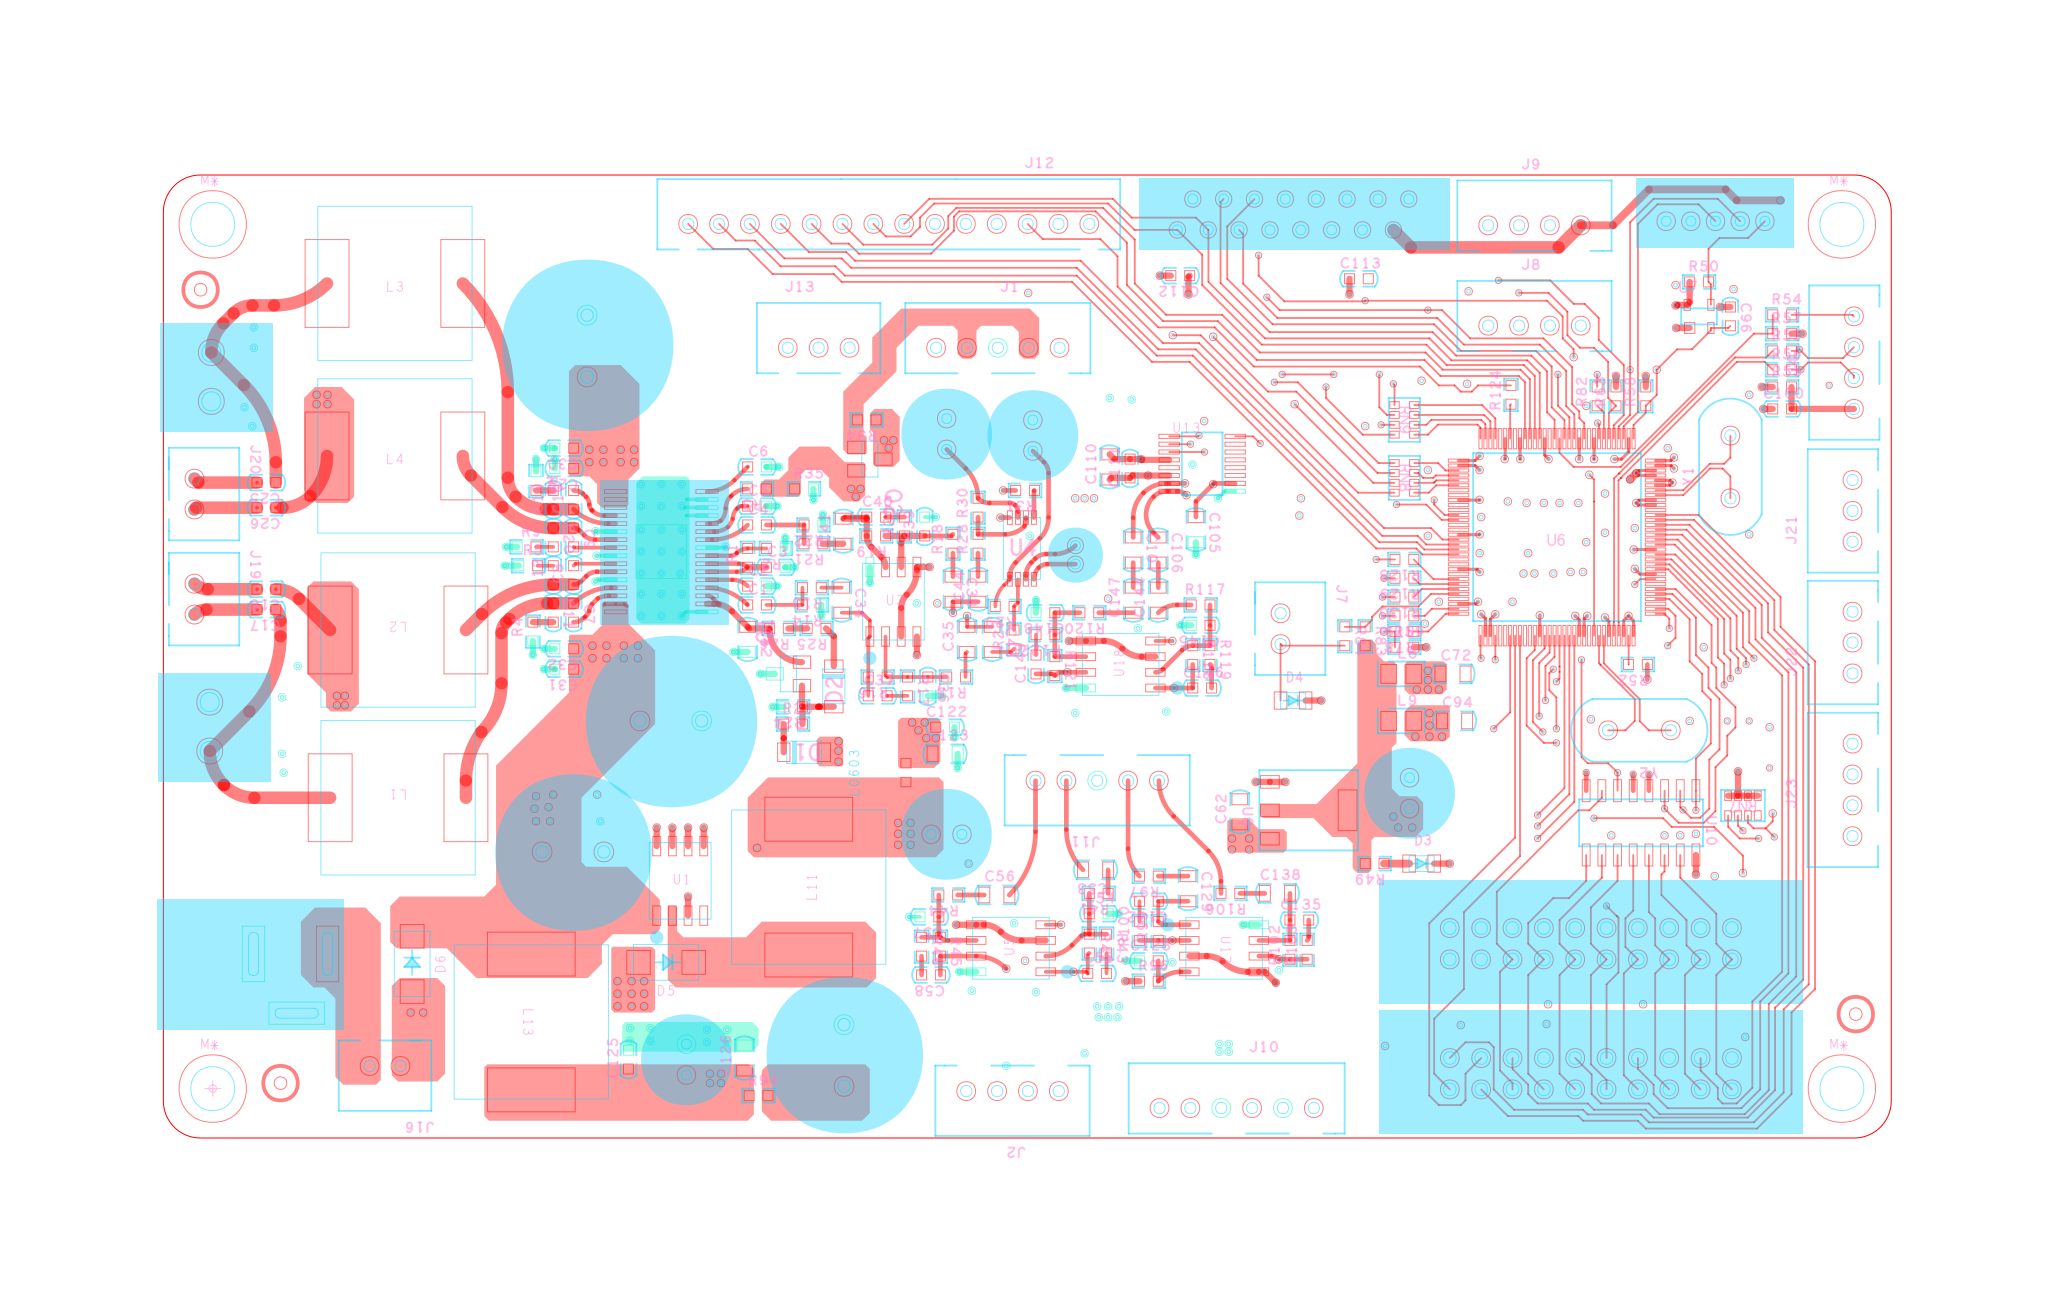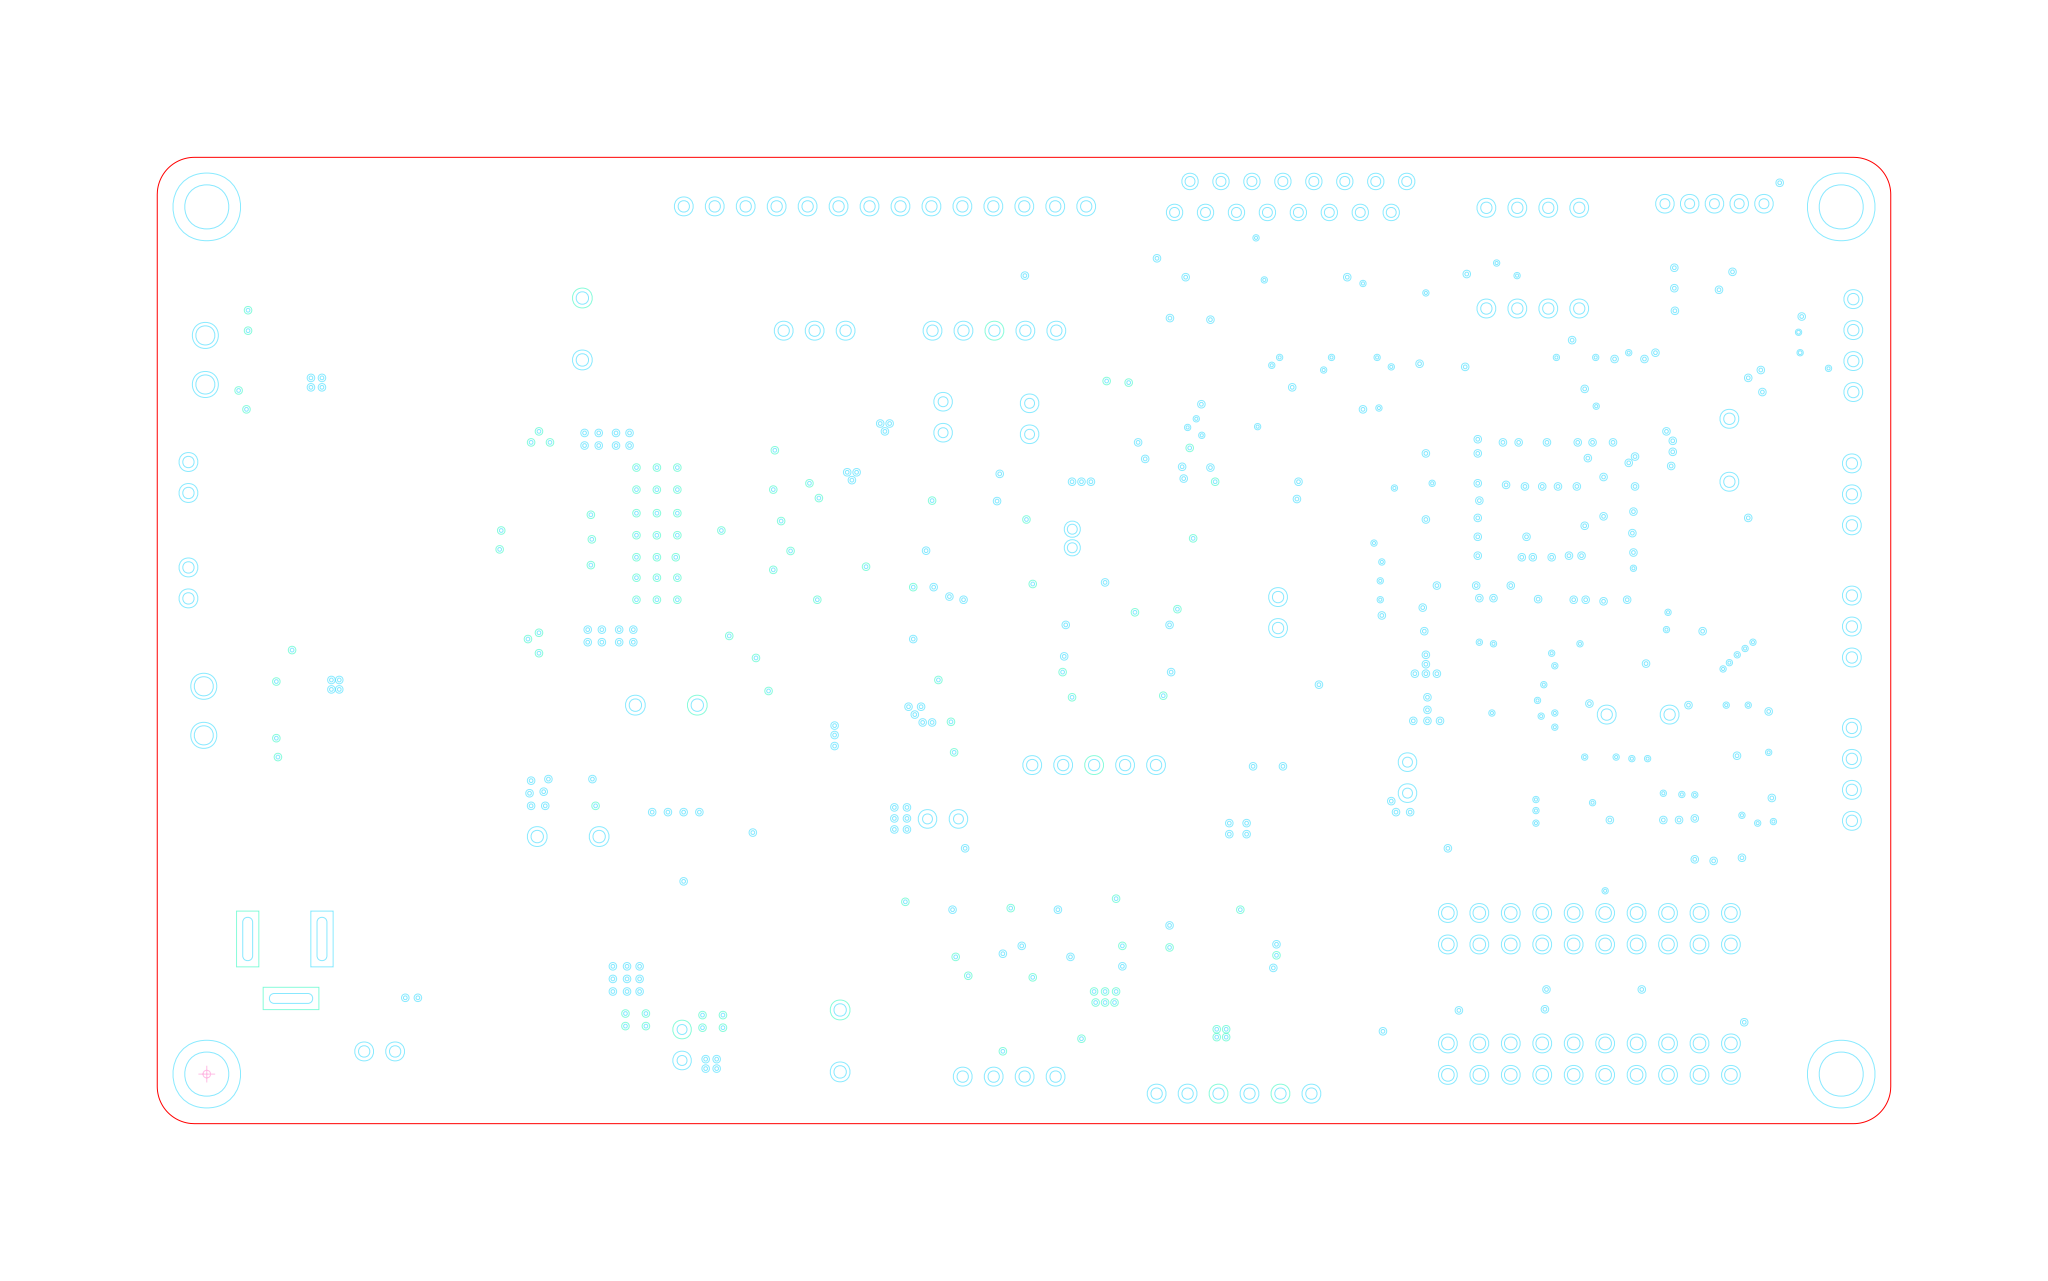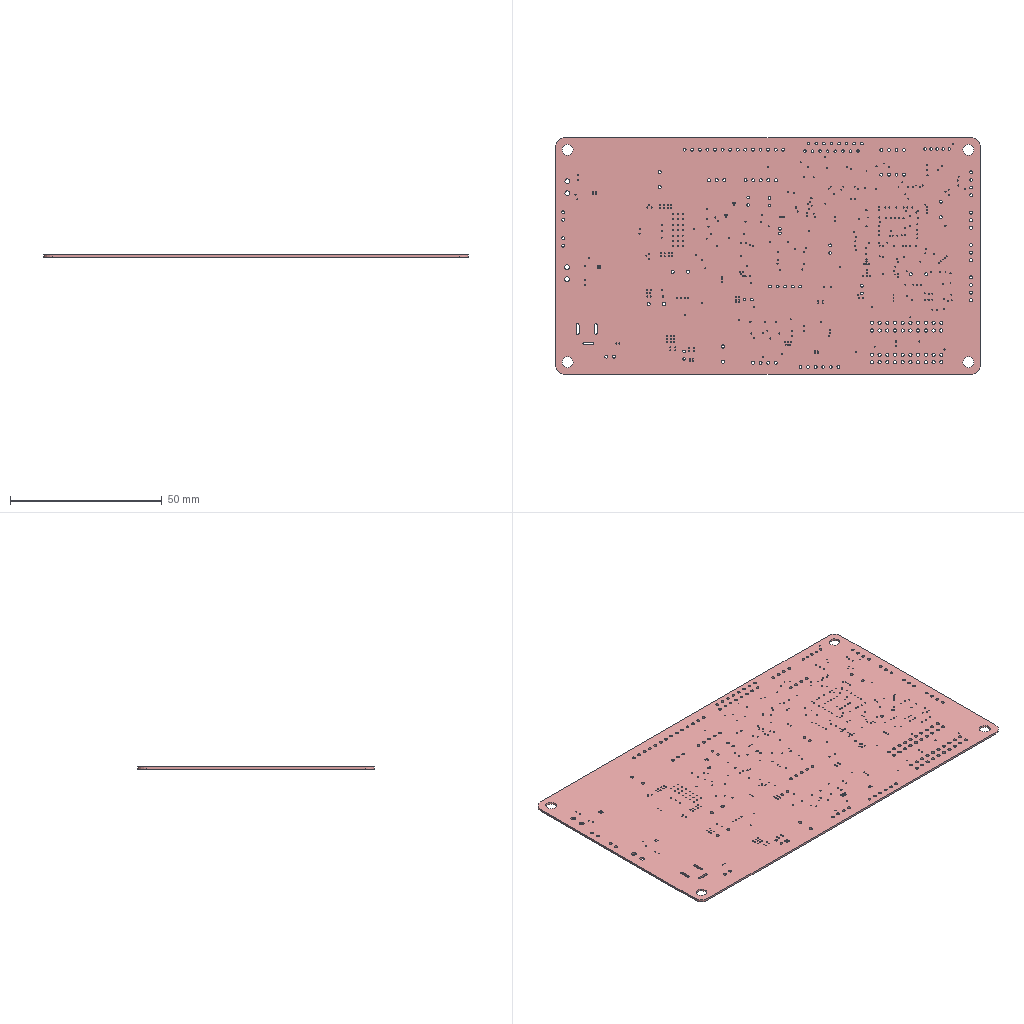Circuit board layout | Cadence Allegro | box 140 x 78 x 0.7 mm
Layer stack:
# Cadence Allegro layer stack of  (unit mm; from the constraint file cross-section; dielectric type: 0 not recorded (Allegro does not mark core vs prepreg), 3 surface material)
index,name,kind,layer,copper_thickness_mm,dielectric_type,dielectric_thickness_mm,dielectric_material,dielectric_constant
0,Top Surface,other,,,,,,
1,TOP,copper,TOP,0.0305,,,,
2,Dielectric1,dielectric,,,0,0.2032,FR-4,4.5
3,L2GND,copper,L2GND,0.0305,,,,
4,Dielectric2,dielectric,,,0,0.2032,FR-4,4.5
5,L3VCC,copper,L3VCC,0.0305,,,,
6,Dielectric3,dielectric,,,0,0.2032,FR-4,4.5
7,BOTTOM,copper,BOTTOM,0.0305,,,,
8,Bottom Surface,other,,,,,,
# drill layer pairs: low layer,high layer
drill_pair,TOP,BOTTOM
Part placement:
REFDES,COMP_VALUE,SYM_NAME,SYM_X,SYM_Y,SYM_ROTATE,SYM_MIRROR
C1,1nF,C0603,1736.220,1542.520,0.000,NO
C2,1nF,C0603,1736.220,1602.520,0.000,NO
C3,1nF,C0603,1796.220,1662.520,0.000,NO
C4,1nF,C0603,1736.220,1797.520,0.000,NO
C5,1nF,C0603,1736.220,1857.520,0.000,NO
C6,1nF,C0603,1736.220,1982.520,0.000,NO
C7,220nF/50V,C0603,1151.220,1517.520,270.000,NO
C8,220nF/50V,C0603,1151.220,1637.520,90.000,NO
C9,220nF/50V,C0603,1151.220,1757.520,270.000,NO
C10,220nF/50V,C0603,1151.220,1877.520,90.000,NO
C11,33pF/50V,C0603,1086.220,1517.520,270.000,NO
C12,33pF/50V,C0603,1086.220,1637.520,90.000,NO
C13,680nF,C0603,256.220,1097.520,90.000,YES
C14,680nF,C0603,256.220,1217.520,90.000,YES
C15,10nF/50V,C0603,301.220,1007.520,0.000,YES
C16,10nF/50V,C0603,301.220,1307.520,0.000,YES
C17,DNP-3.3uF/50V,C0603,171.220,1527.520,180.000,NO
C18,DNP-3.3uF/50V,C0603,171.220,1592.520,180.000,NO
C19,33pF/50V,C0603,1086.220,1877.520,90.000,NO
C20,33pF/50V,C0603,1086.220,1757.520,270.000,NO
C21,680nF,C0603,166.220,2332.520,270.000,YES
C22,680nF,C0603,166.220,2202.520,270.000,YES
C23,10nF/50V,C0603,196.220,2427.520,0.000,YES
C24,10nF/50V,C0603,196.220,2112.520,0.000,YES
C25,DNP-3.3uF/50V,C0603,171.220,1932.520,180.000,NO
C26,DNP-3.3uF/50V,C0603,171.220,1852.520,180.000,NO
C27,1000uF/35V,CAP_13X20MM,1194.251,2367.914,90.000,NO
C28,1000uF/35V,CAP_13X20MM,1461.220,1172.520,0.000,NO
C29,0.1uF,C0603,1121.220,1977.520,180.000,NO
C30,0.1uF,C0603,1121.220,2042.520,180.000,NO
C31,1nF,C0603,1121.220,1337.520,180.000,NO
C32,1nF,C0603,1121.220,1402.520,180.000,NO
C33,0.1uF,C0603,2246.220,1472.520,90.000,YES
C34,10uF,C0805,2006.220,1557.520,270.000,NO
C35,10uF,C0805,2406.220,1432.520,90.000,NO
C36,1nF,C0603,2281.220,1282.520,270.000,NO
C37,100pF,C0603,2121.220,1252.520,0.000,NO
C38,10uF,C0805,2361.220,1592.520,270.000,NO
C39,1nF,C0603,2271.220,1792.520,90.000,NO
C40,100pF,C0603,2116.220,1822.520,0.000,NO
C41,10uF,C0805,2011.220,1777.520,90.000,NO
C42,10uF,C0805,1706.220,1432.520,270.000,NO
C43,10uF,C0805,2486.220,1432.520,270.000,NO
C44,10uF,C0805,2441.220,1592.520,90.000,NO
C45,100uF/10V,CAP_6P3X11MM,2616.220,2082.520,90.000,NO
C46,100uF/10V,CAP_6P3X11MM,2341.220,2087.520,90.000,NO
C47,1uF,C0603,2576.220,1822.520,180.000,YES
C48,4.7uF/35V,CAP_4X7MM,2752.007,1702.126,270.000,NO
C49,0.1uF,C0603,2141.220,1977.520,90.000,YES
C50,10uF,C0805,2531.220,292.520,270.000,YES
C51,0.1uF,C0603,2626.220,527.520,180.000,YES
C52,10uF,C0805,2746.220,287.520,270.000,YES
C53,10uF,C0805,2816.220,697.520,180.000,NO
C54,1nF,C0603,2826.220,557.520,0.000,NO
C55,100pF,C0603,2821.220,367.520,0.000,NO
C56,10uF,C0805,2501.220,617.520,0.000,NO
C57,1nF,C0603,2286.220,547.520,180.000,NO
C58,100pF,C0603,2291.220,362.520,180.000,NO
C59,DNP,C0603,2716.220,112.520,180.000,YES
C60,DNP,C0603,2501.220,112.520,180.000,YES
C61,0.1uF,C0603,3276.220,877.520,270.000,YES
C62,10uF,C0805,3276.220,882.520,90.000,NO
C63,0.1uF,C0603,3921.220,937.520,270.000,YES
C64,100uF,CAP_6P3X11MM,3817.795,942.126,90.000,NO
C65,0.1uF,C0603,4131.220,1937.520,90.000,YES
C66,10nF,C0603,4356.220,1937.520,90.000,YES
C67,10uF,C0805,3981.220,1597.520,0.000,YES
C68,0.1uF,C0603,4296.220,1937.522,90.000,YES
C69,10nF,C0603,4081.220,1992.520,270.000,YES
C70,0.1uF,C0603,3956.220,1322.520,180.000,YES
C71,10nF,C0603,4081.220,1852.520,90.000,YES
C72,10uF,C0805,3956.220,1322.520,0.000,NO
C73,0.1uF,C0603,4001.220,1737.520,90.000,YES
C74,10uF,C0805,4651.220,1747.520,270.000,YES
C75,0.1uF,C0603,4246.220,1937.520,90.000,YES
C76,10nF,C0603,4591.220,1997.520,180.000,YES
C77,0.1uF,C0603,4191.220,1937.520,90.000,YES
C78,10nF,C0603,4116.220,1587.520,180.000,YES
C79,0.1uF,C0603,4471.220,1742.520,0.000,YES
C80,0.1uF,C0603,4276.220,1577.520,270.000,YES
C81,10nF,C0603,4331.220,1577.520,270.000,YES
C82,10uF,C0805,4121.220,1707.520,180.000,YES
C83,0.1uF,C0603,4116.220,1642.520,180.000,YES
C84,10nF,C0603,4591.220,1917.520,180.000,YES
C85,10uF,C0805,4581.220,1747.520,270.000,YES
C86,10uF,C0805,4451.220,1672.520,0.000,YES
C87,0.1uF,C0603,4386.220,1577.520,270.000,YES
C88,0.1uF,C0603,4451.220,2052.520,180.000,YES
C89,10nF,C0603,4471.220,1867.520,0.000,YES
C90,0.1uF,C0603,4471.220,1807.520,0.000,YES
C91,0.1uF,C0603,4216.220,1577.520,270.000,YES
C92,0.1uF,C0603,4696.220,1997.520,270.000,YES
C93,0.1uF,C0603,4441.220,1577.520,270.000,YES
C94,10uF,C0805,3961.220,1172.520,0.000,NO
C95,0.1uF,C0603,4066.220,1472.520,180.000,YES
C96,0.1uF,C0603,4841.220,2462.520,270.000,NO
C97,0.1uF,C0603,4701.220,2462.520,90.000,YES
C98,0.1uF,C0603,4781.220,2612.520,270.000,YES
C99,10uF,C0805,4711.220,2602.520,90.000,YES
C100,0.1uF,C0603,5006.220,2167.520,0.000,NO
C101,0.1uF,C0603,4761.220,642.520,0.000,YES
C102,0.1uF,C0603,4966.220,1087.520,90.000,YES
C103,10uF,C0805,2861.220,2127.520,270.000,YES
C104,0.1uF,C0603,2931.220,2127.520,270.000,YES
C105,10uF,C0805,3136.220,1782.520,270.000,NO
C106,10uF,C0805,3016.220,1717.520,270.000,NO
C107,10uF,C0805,2936.220,1717.520,270.000,NO
C108,10uF,C0805,2862.535,1982.520,270.000,YES
C109,0.1uF,C0603,2927.535,1977.520,270.000,YES
C110,10uF,C0805,2861.220,1982.520,90.000,NO
C111,0.1uF,C0603,2926.220,1977.520,90.000,NO
C112,0.1uF,C0603,3086.220,2592.520,180.000,NO
C113,0.1uF,C0603,3656.220,2582.520,0.000,NO
C114,0.1uF,C0603,3846.220,1707.520,0.000,YES
C115,22pF,C0603,4871.220,1797.520,180.000,YES
C116,22pF,C0603,4871.220,2172.520,180.000,YES
C117,22pF,C0603,4681.220,1217.520,180.000,YES
C118,22pF,C0603,4416.220,1217.520,0.000,YES
C119,1nF/35V,C0603,1156.220,937.520,180.000,YES
C120,0.1uF,C0603,2341.220,717.520,180.000,YES
C121,0.1uF,C0603,2542.106,682.520,90.000,YES
C122,0.1uF,C0603,2336.220,1152.520,0.000,NO
C123,10uF,C0805,2336.220,1067.520,0.000,NO
C124,10uF/35V,C0805,1156.220,852.520,180.000,YES
C125,0.1uF/35V,C0603,1326.220,92.520,90.000,NO
C126,10uF/35V,C0805,1696.220,97.520,90.000,NO
C127,0.1uF/35V,C0603,2131.220,37.520,270.000,YES
C128,0.1uF,C0603,2986.220,407.520,0.000,NO
C129,10uF,C0805,3111.220,637.520,270.000,NO
C130,10uF,C0805,3146.220,317.520,0.000,YES
C131,1nF,C0603,3126.220,422.520,90.000,YES
C132,100pF,C0603,2986.220,597.520,180.000,NO
C133,10uF,C0805,3296.220,312.520,180.000,YES
C134,1nF,C0603,3321.220,422.520,90.000,YES
C135,100pF,C0603,3466.220,537.520,0.000,NO
C138,10uF,C0805,3396.220,622.520,0.000,NO
C139,100pF,C0603,3151.220,182.520,180.000,YES
C140,100pF,C0603,3286.220,182.520,0.000,YES
C141,10uF,C0805,2811.220,1277.520,0.000,YES
C142,0.1uF,C0603,2981.220,1427.520,180.000,YES
C143,10uF,C0805,2986.220,1277.520,180.000,YES
C144,10uF,C0805,3016.220,1557.520,90.000,NO
C145,1nF,C0603,3151.220,1477.520,180.000,NO
C146,100pF,C0603,3156.220,1277.520,0.000,NO
C147,10uF,C0805,2936.220,1557.520,90.000,NO
C148,1nF,C0603,2656.220,1517.520,180.000,NO
C149,100pF,C0603,2626.220,1352.520,90.000,NO
C150,100uF/35V,CAP_6P3X11MM,1511.220,92.520,90.000,NO
C151,180UF/35V,CAP_6P3X11MM,2340.826,810.945,0.000,NO
C152,470UF/35V,CAP_10X17MM,1149.133,754.882,0.000,NO
C153,470UF/35V,CAP_10X17MM,2013.858,105.434,90.000,NO
D1,IN4148,SOD-123,1886.220,1072.520,180.000,NO
D2,IN4148,SOD-123,1981.220,1282.520,90.000,NO
D3,LED,LED0805,3856.220,717.520,0.000,NO
D4,LED,LED0805,3446.220,1237.520,0.000,NO
D5,SM2150A,SMA-FL,1446.220,402.516,0.000,NO
D6,SS24,DO-214AC_5P28X2P9M,636.220,397.520,90.000,NO
J1,XH_5x1,XH-5A,2701.220,2362.520,0.000,NO
J2,CONN_RCA_2x1,XH-4A,2403.582,-7.952,180.000,NO
J3,PH5x1,PH-5A,4793.779,2765.941,0.000,NO
J4,XH4x1,XH-4A,5235.276,2462.796,90.000,NO
J5,LEFT KEYBOARD,IDC10X2,4396.137,462.008,180.000,NO
J6,RIGHT KEYBOARD,IDC10X2,4396.220,47.520,180.000,NO
J7,XH2x1,XH-2A,3406.220,1417.520,270.000,NO
J8,XH4x1,XH254_4_V,4363.858,2432.992,0.000,NO
J9,XH4x1,XH254_4_V,4363.858,2752.992,0.000,NO
J10,XH6x1,XH-6A,3512.283,-62.008,0.000,NO
J11,XH5x1,XH-5A,2624.566,982.048,180.000,NO
J12,XH14x1,XH254_14_V,2796.220,2757.520,0.000,NO
J13,XH3x1,XH-3A,2031.220,2362.520,0.000,NO
J14,AFC25-S16HCC,FPC_1P25MM16P,3446.220,2787.520,0.000,NO
J15,DC12-24V,DC-0055P5-2P0MM,-165.197,429.410,270.000,NO
J16,XH2x1,XH-2A,500.433,72.048,180.000,NO
J17,VH2x1,VH-2A,-9.528,1154.489,90.000,NO
J18,VH2x1,VH-2A,-4.528,2269.489,90.000,NO
J19,DNP-XH_2x1,XH-2A,-58.308,1511.733,270.000,NO
J20,DNP-XH_2x1,XH-2A,-58.308,1846.733,270.000,NO
J21,XH3x1,XH-3A,5230.748,1940.807,90.000,NO
J22,XH3x1,XH-3A,5230.748,1520.807,90.000,NO
J23,XH4x1,XH254_4_V,5230.748,1100.158,90.000,NO
L1,33uH,L_12P5X12P5X7P5MM,591.220,927.520,180.000,NO
L2,33uH,L_12P5X12P5X7P5MM,591.220,1462.520,180.000,NO
L3,33uH,L_12P5X12P5X7P5MM,581.220,2567.520,0.000,NO
L4,33uH,L_12P5X12P5X7P5MM,581.220,2017.520,0.000,NO
L5,BLM21PG600SN1D,L0603,2406.220,142.520,90.000,YES
L6,BLM21PG600SN1D,L0603,2601.220,147.520,90.000,YES
L7,BLM21PG600SN1D,L0603,2851.220,147.520,90.000,YES
L8,BLM21PG600SN1D,L0805,3791.220,1322.520,0.000,NO
L9,BLM21PG600SN1D,L0805,3791.220,1172.520,0.000,NO
L10,BLM21PG600SN1D,L0805,2776.220,1982.520,270.000,YES
L11,SLF12575T-68uH_2A,L_12P5X12P5X7P5MM,1901.220,642.520,90.000,NO
L12,BLM18PG121SN1D,L0603,2211.220,1007.520,90.000,NO
L13,SLF12575T-68uH_2A,L_12P5X12P5X7P5MM,1016.220,212.520,270.000,NO
L14,4.7uH,L0805,5096.220,1062.520,0.000,YES
L15,4.7uH,L0805,5096.220,952.520,0.000,YES
L16,4.7uH,L0805,5096.220,852.520,0.000,YES
Q1,PMBT3906,SOT-23,1836.220,1322.520,90.000,NO
Q2,PMBT3904,SOT-23,2096.220,2007.520,270.000,NO
R1,100K,R0603,1706.220,1692.520,90.000,NO
R2,20K,R0603,1796.220,1722.520,180.000,NO
R3,49K,R0603,1736.220,1912.520,180.000,NO
R4,10,R0603,1021.220,1457.520,90.000,NO
R5,10,R0603,1006.220,1667.520,0.000,NO
R6,3.3,R0603,331.220,1097.520,270.000,YES
R7,3.3,R0603,331.220,1217.520,90.000,YES
R8,10,R0603,1031.220,1937.520,270.000,NO
R9,10,R0603,1001.220,1727.520,0.000,NO
R10,3.3,R0603,226.220,2332.520,90.000,YES
R11,3.3,R0603,226.220,2202.520,270.000,YES
R12,10,R0603,2311.220,1472.520,90.000,YES
R13,220,R0603,1911.220,1597.520,180.000,NO
R14,47K,R0603,1911.220,1542.520,180.000,NO
R15,6.8K,R0603,2371.220,1312.520,180.000,NO
R16,20K,R0603,2121.220,1312.520,180.000,NO
R17,4.7K,R0603,2216.220,1282.520,270.000,NO
R18,6.8K,R0603,2361.220,1737.520,90.000,NO
R19,20K,R0603,2116.220,1762.520,180.000,NO
R20,4.7K,R0603,2206.220,1792.520,90.000,NO
R21,220,R0603,1916.220,1737.520,180.000,NO
R22,47K,R0603,1916.220,1797.520,180.000,NO
R23,10K,R0603,1851.220,1162.520,0.000,NO
R24,4.7K,R0603,1851.220,1217.520,180.000,NO
R25,100K,R0603,1926.220,1467.520,180.000,NO
R26,100K,R0603,1806.220,1467.520,180.000,NO
R27,20K,R0603,2556.220,1432.520,90.000,NO
R28,20K,R0603,2441.220,1737.520,90.000,NO
R29,20K,R0603,2526.220,1537.520,180.000,NO
R30,20K,R0603,2441.220,1852.520,90.000,NO
R31,100K,R0603,2591.220,1907.520,180.000,NO
R32,10K,R0603,2276.220,2242.520,180.000,YES
R33,10K,R0603,2731.220,2237.520,0.000,YES
R34,100K,R0603,2086.220,2132.520,180.000,NO
R35,47K,R0603,1886.220,1912.520,0.000,NO
R36,220,R0603,2501.220,172.520,0.000,YES
R38,10,R0603,2656.220,437.520,270.000,YES
R39,220,R0603,2716.220,177.520,0.000,YES
R41,6.8K,R0603,2826.220,622.520,180.000,NO
R42,20K,R0603,2796.220,462.520,270.000,NO
R43,4.7K,R0603,2851.220,462.520,270.000,NO
R44,6.8K,R0603,2346.220,617.520,180.000,NO
R45,20K,R0603,2321.220,452.520,270.000,NO
R46,4.7K,R0603,2261.220,452.520,270.000,NO
R47,10K,R0603,2666.220,277.520,270.000,YES
R48,10K,R0603,2456.220,282.520,270.000,YES
R49,4.7K,R0603,3706.220,717.520,180.000,NO
R50,10K,R0603,4741.220,2572.520,0.000,NO
R51,10K,R0603,4851.220,2612.520,90.000,YES
R52,12K,1%,R0603,4546.220,1352.520,180.000,NO
R53,0,R0603,5006.220,2237.520,0.000,NO
R54,4.7K,R0603,5006.220,2467.520,0.000,NO
R55,10,R0603,5006.220,2352.520,0.000,NO
R56,10,R0603,5006.220,2292.520,0.000,NO
R57,10K,R0603,5006.220,2407.520,0.000,NO
R58,10K,R0603,4571.220,2207.520,90.000,NO
R59,10K,R0603,3801.220,1407.520,0.000,NO
R60,10K,R0603,3801.220,1507.520,180.000,YES
R61,10K,R0603,4716.220,1437.520,90.000,YES
R62,10K,R0603,4416.220,2207.520,90.000,YES
R63,10K,R0603,4476.220,2207.520,90.000,NO
R64,1K,R0603,4526.220,807.520,180.000,YES
R65,1K,R0603,4526.220,867.520,180.000,YES
R66,1K,R0603,4526.220,922.520,180.000,YES
R67,1K,R0603,4431.220,952.520,270.000,YES
R68,2.2k,R0603,4011.220,232.520,90.000,YES
R69,2.2k,R0603,3946.220,232.520,90.000,YES
R70,10K,R0603,4831.220,1092.520,270.000,YES
R71,10K,R0603,4901.220,1092.520,270.000,YES
R72,0,R0603,2871.220,2327.520,90.000,YES
R73,10K,R0603,3406.220,1827.520,0.000,YES
R74,10K,R0603,3406.220,1767.520,0.000,YES
R75,10K,R0603,2901.220,1862.520,180.000,YES
R76,10K,R0603,3406.220,1882.520,180.000,YES
R77,10,R0603,4576.220,1412.520,0.000,YES
R78,10,R0603,3801.220,1457.520,180.000,NO
R79,10,R0603,3801.220,1507.520,180.000,NO
R80,10,R0603,4576.220,1467.520,0.000,YES
R81,10,R0603,4401.220,1457.520,0.000,YES
R82,10,R0603,4416.220,2207.520,90.000,NO
R83,10K,R0603,3676.220,1442.520,270.000,NO
R84,1K,R0603,3611.220,1442.520,270.000,NO
R85,1M,R0603,4761.220,1987.520,270.000,YES
R86,1M,R0603,4551.220,1217.520,0.000,YES
R87,10K,R0603,4001.220,2312.520,270.000,YES
R88,10,R0603,4066.220,2312.520,270.000,YES
R89,10,R0603,4166.220,2307.520,270.000,YES
R90,10K,R0603,4006.220,2607.520,270.000,YES
R91,10,R0603,4066.220,2607.520,270.000,YES
R92,10,R0603,4166.220,2612.520,270.000,YES
R93,0,R0603,2476.220,682.520,90.000,YES
R94,10K,R0603,1741.220,-22.480,0.000,NO
R95,10K,R0603,2216.220,37.520,90.000,YES
R96,10,R0603,2986.220,342.520,0.000,NO
R97,1K,R0603,2986.220,677.520,180.000,NO
R98,10K,R0603,3186.220,422.520,270.000,YES
R99,12K,R0603,3016.220,502.520,90.000,NO
R100,4.7K,R0603,2956.220,502.520,90.000,NO
R101,10K,R0603,3256.220,422.520,270.000,YES
R102,12K,R0603,3436.220,442.520,90.000,NO
R103,4.7K,R0603,3491.220,442.520,90.000,NO
R106,1K,R0603,3246.220,622.520,180.000,NO
R107,1K,R0603,3121.220,77.520,270.000,YES
R108,4.7K,R0603,3151.220,242.520,0.000,YES
R109,1K,R0603,3316.220,77.520,270.000,YES
R110,4.7K,R0603,3286.220,242.520,180.000,YES
R111,0,R0603,3021.220,212.520,90.000,YES
R112,220,R0603,2851.220,1167.520,90.000,YES
R113,47K,R0603,2791.220,1167.520,90.000,YES
R114,10,R0603,2981.220,1512.520,180.000,YES
R115,220,R0603,2946.220,1172.520,90.000,YES
R116,47K,R0603,3006.220,1172.520,90.000,YES
R117,6.8K,R0603,3151.220,1542.520,0.000,NO
R118,20K,R0603,3126.220,1382.520,270.000,NO
R119,4.7K,R0603,3181.220,1382.520,270.000,NO
R120,6.8K,R0603,2796.220,1517.520,180.000,NO
R121,20K,R0603,2686.220,1347.520,270.000,NO
R122,4.7K,R0603,2656.220,1447.520,180.000,NO
R123,1K,R0603,2601.220,2602.520,270.000,YES
R124,10,R0603,4141.220,2212.520,90.000,NO
R125,1K,R0603,2501.220,2597.520,90.000,YES
R126,1K,R0603,2406.220,2597.520,90.000,YES
R127,1K,R0603,2301.220,2597.520,90.000,YES
R128,10,R0603,3801.220,1687.520,180.000,NO
R129,10,R0603,3801.220,1627.520,180.000,NO
R130,10,R0603,3801.220,1567.520,180.000,NO
R131,0,R0603,1546.220,657.520,180.000,YES
R133,470,R0603,5076.220,1812.520,90.000,YES
R134,470,R0603,5066.220,1392.520,90.000,YES
RN2,2.2k,RN0603,4841.220,237.520,180.000,YES
RN3,2.2k,RN0603,4171.220,237.520,180.000,YES
RN4,2.2k,RN0603,3771.220,42.520,90.000,YES
RN5,2.2k,RN0603,4656.220,237.520,0.000,YES
RN6,2.2k,RN0603,4341.220,237.520,0.000,YES
RN7,10k,RN0603,4881.220,902.520,0.000,NO
RN8,10,RN0603,3801.220,1947.520,90.000,NO
RN9,10,RN0603,3801.220,2132.520,90.000,NO
U1,XL1509-5.0,SO8,1491.220,662.520,0.000,NO
U2,TPA3118D2,DAP-32,1430.984,1712.244,180.000,NO
U3,NJM4580E,SO8,2171.220,1552.520,0.000,NO
U4,LM4809MM,TSSOP8_0P65M_3X5M,2581.220,1722.520,0.000,NO
U5,NJM4580E,SO8,2546.220,447.520,90.000,NO
U6,SAM5704B,LQFP128_P40,4288.220,1758.520,270.000,NO
U7,MAX811TEUS+T,SOT143_4,4741.220,2462.520,0.000,NO
U8,LM1117S-3.3,SOT223_4,3496.220,887.520,270.000,NO
U9,ESD05V14T-LC,SOT143_4,5126.574,2322.540,0.000,YES
U10,74HC238,SOIC16,4556.220,847.520,270.000,NO
U11,74HCT4051,SOIC16,4806.220,847.520,270.000,YES
U12,AK4388AET,TSSOP16,3166.220,1967.520,0.000,YES
U13,PCM1754DBQR,SSOP16,3156.220,1992.520,0.000,NO
U14,MX25L25635FMI-10G,MX25L25635FMI-10G,3237.476,2387.520,90.000,YES
U15,MX25L25635FMI-10G,MX25L25635FMI-10G,3751.220,2387.520,90.000,YES
U16,AT45DB041E,SO8,3851.220,1922.520,180.000,YES
U17,NJM4580E,SO8,3226.220,447.520,270.000,NO
U18,NJM4580E,SO8,2896.220,1352.520,90.000,NO
Y1,12.288M,XTALT_49S,4841.220,1882.520,90.000,NO
Y2,12M,XTALT_49S,4651.220,1142.520,180.000,NO
Pad and via stacks:
# Allegro (Cadence) via spans and padstacks; design units: ("mils" 3 1000)
# via spans: padstack,start_layer,end_layer,net_example,count
VIA1220,ETCH/TOP,ETCH/BOTTOM,N50849,2
VIA10_F,ETCH/TOP,ETCH/BOTTOM,BCK,65
VIA24D12A34,ETCH/TOP,ETCH/BOTTOM,AGND,327
# Allegro padstack definitions: name,start_layer,end_layer,drill,plating,holeType,type
S80X70S,"ETCH/TOP","ETCH/TOP",0.0,"PLATED","none","smd"
S60X50S,"ETCH/TOP","ETCH/TOP",0.0,"PLATED","none","smd"
S32S,"ETCH/TOP","ETCH/TOP",0.0,"PLATED","none","smd"
S65X10S_3M,"ETCH/TOP","ETCH/TOP",0.0,"PLATED","none","smd"
S70X25S,"ETCH/TOP","ETCH/TOP",0.0,"NON_PLATED","none","smd"
S60X40S,"ETCH/TOP","ETCH/TOP",0.0,"PLATED","none","smd"
S130X60S,"ETCH/TOP","ETCH/TOP",0.0,"PLATED","none","smd"
S50X40S,"ETCH/TOP","ETCH/TOP",0.0,"PLATED","none","smd"
STP_C40,"ETCH/TOP","ETCH/TOP",0.0,"PLATED","none","smd"
S76X25S,"ETCH/TOP","ETCH/TOP",0.0,"PLATED","none","smd"
S35X20S,"ETCH/TOP","ETCH/TOP",0.0,"PLATED","none","smd"
S35X33S,"ETCH/TOP","ETCH/TOP",0.0,"PLATED","none","smd"
S30X22S,"ETCH/TOP","ETCH/TOP",0.0,"PLATED","none","smd"
S40X30S,"ETCH/TOP","ETCH/TOP",0.0,"PLATED","none","smd"
S110X40S,"ETCH/TOP","ETCH/TOP",0.0,"PLATED","none","smd"
S120X55S,"ETCH/TOP","ETCH/TOP",0.0,"PLATED","none","smd"
S50X35S,"ETCH/TOP","ETCH/TOP",0.0,"PLATED","none","smd"
P60C36C,"ETCH/TOP","ETCH/BOTTOM",36.0,"PLATED","circle_drill","through"
P60S36C,"ETCH/TOP","ETCH/BOTTOM",36.0,"PLATED","circle_drill","through"
VIA1220,"ETCH/TOP","ETCH/BOTTOM",12.0,"PLATED","circle_drill","through"
P48C28C,"ETCH/TOP","ETCH/BOTTOM",28.0,"PLATED","circle_drill","through"
P48S28C,"ETCH/TOP","ETCH/BOTTOM",28.0,"PLATED","circle_drill","through"
MHOLE160,"ETCH/TOP","ETCH/BOTTOM",160.0,"PLATED","circle_drill","through"
P51C31C,"ETCH/TOP","ETCH/BOTTOM",31.0,"PLATED","circle_drill","through"
VIA2032,"ETCH/TOP","ETCH/BOTTOM",20.0,"PLATED","circle_drill","through"
S65X13S,"ETCH/TOP","ETCH/TOP",0.0,"PLATED","none","smd"
MHOLE140,"ETCH/TOP","ETCH/BOTTOM",140.0,"PLATED","circle_drill","through"
S225X65S,"ETCH/TOP","ETCH/TOP",0.0,"PLATED","none","smd"
S150X95S,"ETCH/TOP","ETCH/TOP",0.0,"PLATED","none","smd"
SMD32_35,"ETCH/TOP","ETCH/TOP",0.0,"PLATED","none","smd"
SMD30_32,"ETCH/TOP","ETCH/TOP",0.0,"PLATED","none","smd"
SMD0R76X0R80,"ETCH/TOP","ETCH/TOP",0.0,"PLATED","none","smd"
R40X55,"ETCH/TOP","ETCH/TOP",0.0,"PLATED","none","smd"
SMD1R00X1R50,"ETCH/TOP","ETCH/TOP",0.0,"PLATED","none","smd"
SMD35_32,"ETCH/TOP","ETCH/TOP",0.0,"PLATED","none","smd"
SMD45_50,"ETCH/TOP","ETCH/TOP",0.0,"PLATED","none","smd"
SMD2R16X2R74,"ETCH/TOP","ETCH/TOP",0.0,"PLATED","none","smd"
SMD40_50,"ETCH/TOP","ETCH/TOP",0.0,"PLATED","none","smd"
R62X25,"ETCH/TOP","ETCH/TOP",0.0,"PLATED","none","smd"
SMD_REC_2X0R6,"ETCH/TOP","ETCH/TOP",0.0,"PLATED","none","smd"
SMD0R40X1R10,"ETCH/TOP","ETCH/TOP",0.0,"PLATED","none","smd"
R140X280,"ETCH/TOP","ETCH/TOP",0.0,"PLATED","none","smd"
SMD1R00X1R40,"ETCH/TOP","ETCH/TOP",0.0,"PLATED","none","smd"
R75X76,"ETCH/TOP","ETCH/TOP",0.0,"PLATED","none","smd"
R180_30,"ETCH/TOP","ETCH/TOP",0.0,"PLATED","none","smd"
R411_436,"ETCH/TOP","ETCH/TOP",0.0,"PLATED","none","smd"
P100C36C,"ETCH/TOP","ETCH/BOTTOM",40.157,"PLATED","circle_drill","through"
P100C80C,"ETCH/TOP","ETCH/BOTTOM",31.496,"PLATED","circle_drill","through"
P100C210C,"ETCH/TOP","ETCH/BOTTOM",60.63,"PLATED","circle_drill","through"
R350X180,"ETCH/TOP","ETCH/BOTTOM",31.496,"PLATED","oval slot","through"
P100C88C,"ETCH/TOP","ETCH/BOTTOM",31.496,"PLATED","circle_drill","through"
P100C100C,"ETCH/TOP","ETCH/BOTTOM",39.37,"PLATED","circle_drill","through"
P100C75C,"ETCH/TOP","ETCH/BOTTOM",31.496,"PLATED","circle_drill","through"
R34X37,"ETCH/TOP","ETCH/TOP",0.0,"NON_PLATED","none","smd"
VIA10_F,"ETCH/TOP","ETCH/BOTTOM",10.0,"PLATED","circle_drill","through"
VIA24D12A34,"ETCH/TOP","ETCH/BOTTOM",12.0,"PLATED","circle_drill","through"
ID-BOARD,"ETCH/TOP","ETCH/TOP",0.0,"PLATED","none","smd"
Design rules, without the lines most boards share, first 14 of 38 lines:
# Cadence Allegro design rules of  (from the Constraint Manager export constraints.dcfx, design unit mil; typed fields in mm)
# columns: name | kind | enabled | priority | scope1 | scope2 | descriptor | typed fields (field=value)
# Allegro precedence (priority 1 wins): 1 Region class-to-class, 2 Region class, 3 Region, 4 class-to-class, 5 DiffPair/Bus/NetGroup override, 6 NetClass, 7 constraint set (CSet) default
# per-layer values are written LAYER=value in the descriptor and LAYER:mm in the typed field; a maximum of 0 means no limit set
# --- net classes (and buses / net groups) ---
15 | NetClass | enabled | 6 | no members | All | Net Class (SpacingCSet=DEFAULT) (members: 0) | spacingcset=DEFAULT
BUS4 | Bus | enabled | 5 | SPI0, SPI1, SPICK | All | Bus (members: 3 Net) |
2 | Bus | enabled | 5 | QNR3, QNR2, QNR1, QNR0 | All | Bus (members: 4 Net) |
1 | Bus | enabled | 5 | QNR7, QNR6, QNR5, QNR4 | All | Bus (members: 4 Net) |
U5U7 | Bus | enabled | 5 | DABD0, MCLK, BCK, LRCK | All | Bus (members: 4 Net) |
# --- track widths, neck and differential-pair gap (physical constraint sets) ---
100OHM | PhysicalCSet | enabled | 7 | not referenced | All | Physical Constraint (Min Line Width=14mil) (Max Line Width=1000mil) (Min Neck Width=5mil) (Max Neck Length=10000mil) (DiffPair Primary Gap=8mil) (DiffPair Neck Gap=0mil) (DiffPair Min Space=1mil) (DiffPair Coupled +Tol=0mil) (DiffPair Coupled -Tol=0mil) (Min BB Via Stagger=5mil) (Max BB Via Stagger=0mil) (T-junctions=ANYWHERE) (Pad-pad direct connect=ALL_ALLOWED) (Allowed vias=VIA1220, VIA2032) | min_line_width=0.3556 min_neck_width=0.127 min_bvia_stagger=0.127 max_bvia_stagger=0 ts_allowed=ANYWHERE diffp_primary_gap=0.2032 diffp_neck_gap=0 max_line_width=25.4 maximum_neck_length=254 pad_pad_direct_connect=ALL_ALLOWED allow_on_etch_subclass=TRUE diffp_coupled_plus=0 diffp_coupled_minus=0 diffp_min_space=0.0254 vias=VIA1220,VIA2032
90OHM | PhysicalCSet | enabled | 7 | DiffPair(1): DP1; Net(4): N50853, N50849, USBDP, USBDM | All | Physical Constraint (Min Line Width=6mil) (Max Line Width=1000mil) (Min Neck Width=5mil) (Max Neck Length=10000mil) (DiffPair Primary Gap=8mil) (DiffPair Neck Gap=0mil) (DiffPair Min Space=1mil) (DiffPair Coupled +Tol=0mil) (DiffPair Coupled -Tol=0mil) (Min BB Via Stagger=5mil) (Max BB Via Stagger=0mil) (T-junctions=ANYWHERE) (Pad-pad direct connect=ALL_ALLOWED) (Allowed vias=VIA1220, VIA2032) | min_line_width=0.1524 min_neck_width=0.127 min_bvia_stagger=0.127 max_bvia_stagger=0 ts_allowed=ANYWHERE diffp_primary_gap=0.2032 diffp_neck_gap=0 max_line_width=25.4 maximum_neck_length=254 pad_pad_direct_connect=ALL_ALLOWED allow_on_etch_subclass=TRUE diffp_coupled_plus=0 diffp_coupled_minus=0 diffp_min_space=0.0254 vias=VIA1220,VIA2032
DEFAULT | PhysicalCSet | enabled | 7 | Design default | All | Physical Constraint (Min Line Width=6mil) (Max Line Width=1000mil) (Min Neck Width=5mil) (Max Neck Length=10000mil) (DiffPair Primary Gap=0mil) (DiffPair Neck Gap=0mil) (DiffPair Min Space=0mil) (DiffPair Coupled +Tol=0mil) (DiffPair Coupled -Tol=0mil) (Min BB Via Stagger=5mil) (Max BB Via Stagger=0mil) (T-junctions=ANYWHERE) (Pad-pad direct connect=ALL_ALLOWED) (Allowed vias=VIA24D12A34, VIA10_F) | min_line_width=0.1524 min_neck_width=0.127 min_bvia_stagger=0.127 max_bvia_stagger=0 ts_allowed=ANYWHERE diffp_primary_gap=0 diffp_neck_gap=0 max_line_width=25.4 maximum_neck_length=254 pad_pad_direct_connect=ALL_ALLOWED allow_on_etch_subclass=TRUE diffp_coupled_plus=0 diffp_coupled_minus=0 diffp_min_space=0 vias=VIA24D12A34,VIA10_F